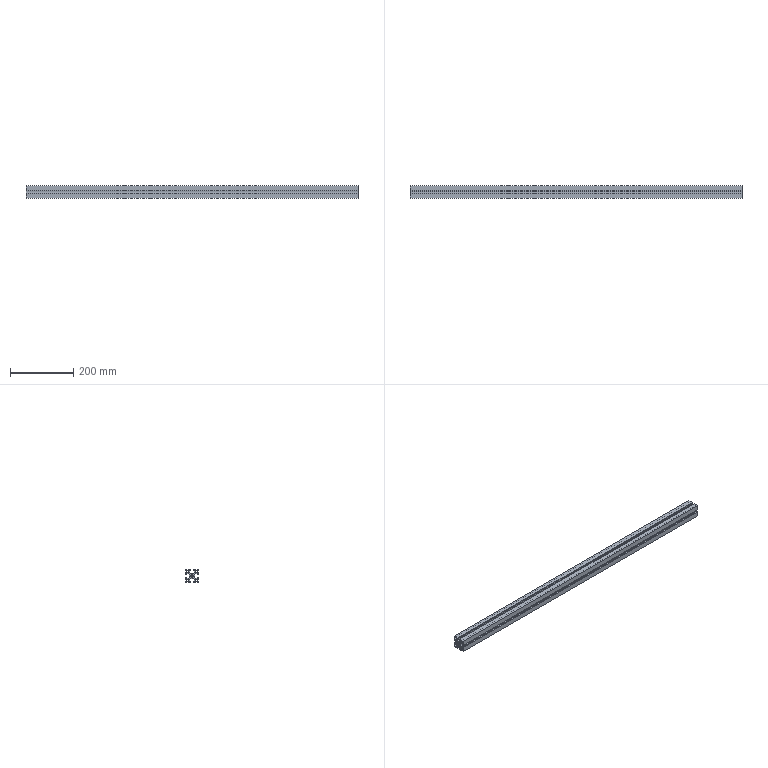Part | STEP file | PN_0024 (upright stop) | 1 solid | 57 faces | box 1050 x 40 x 40 mm | volume 867444 mm3 | plane 34 | cylinder 19 | cone 4 | commonest cylinder face diameters 8 x8 30 x5 6.8 x4 6.7 x2